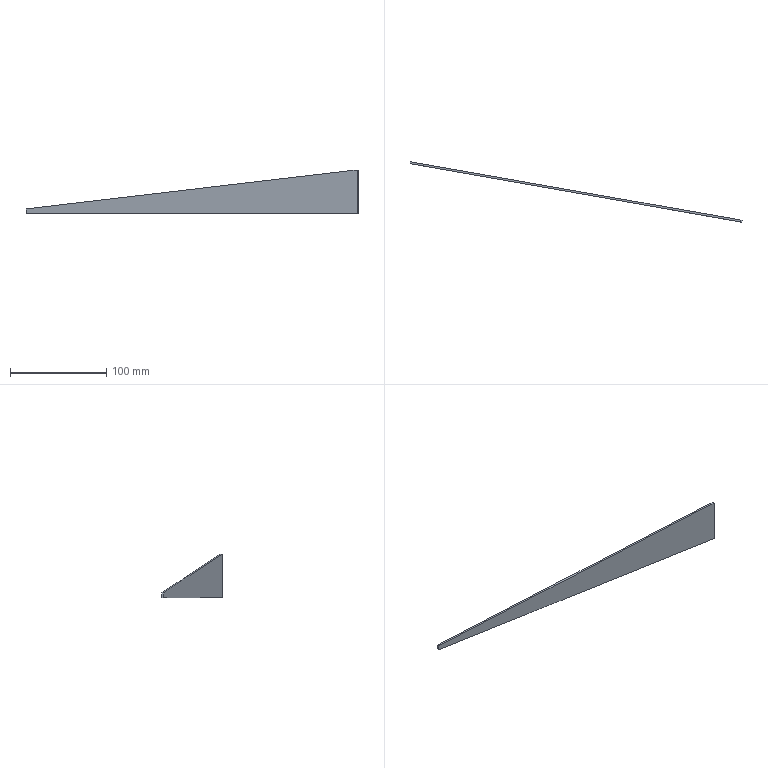Part | SolidWorks | features Extrusion 1 | 1 solid | 7 faces | box 345.03 x 62.746 x 45 mm | volume 17700 mm3 | plane 7
STEP:
#1=CARTESIAN_POINT('',(-12.484,1.186,10.));
#2=VERTEX_POINT('',#1);
#3=CARTESIAN_POINT('',(-357.166,61.963,10.));
#4=VERTEX_POINT('',#3);
#5=CARTESIAN_POINT('',(-12.484,1.186,10.));
#6=DIRECTION('',(-0.9848,0.1736,0.));
#7=VECTOR('',#6,1000.);
#8=LINE('',#5,#7);
#9=EDGE_CURVE('',#2,#4,#8,.T.);
#10=ORIENTED_EDGE('',*,*,#9,.T.);
#11=CARTESIAN_POINT('',(-356.819,63.932,10.));
#12=VERTEX_POINT('',#11);
#13=CARTESIAN_POINT('',(-356.819,63.932,10.));
#14=DIRECTION('',(-0.1736,-0.9848,0.));
#15=VECTOR('',#14,1000.);
#16=LINE('',#13,#15);
#17=EDGE_CURVE('',#12,#4,#16,.T.);
#18=ORIENTED_EDGE('',*,*,#17,.F.);
#19=CARTESIAN_POINT('',(-12.136,3.155,10.));
#20=VERTEX_POINT('',#19);
#21=CARTESIAN_POINT('',(-12.136,3.155,10.));
#22=DIRECTION('',(-0.9848,0.1736,0.));
#23=VECTOR('',#22,1000.);
#24=LINE('',#21,#23);
#25=EDGE_CURVE('',#20,#12,#24,.T.);
#26=ORIENTED_EDGE('',*,*,#25,.F.);
#27=CARTESIAN_POINT('',(-12.136,3.155,10.));
#28=DIRECTION('',(-0.1736,-0.9848,0.));
#29=VECTOR('',#28,1000.);
#30=LINE('',#27,#29);
#31=EDGE_CURVE('',#20,#2,#30,.T.);
#32=ORIENTED_EDGE('',*,*,#31,.T.);
#33=EDGE_LOOP('',(#10,#18,#26,#32));
#34=FACE_OUTER_BOUND('',#33,.T.);
#35=CARTESIAN_POINT('',(-12.136,3.155,10.));
#36=DIRECTION('',(0.,0.,1.));
#37=DIRECTION('',(1.,0.,0.));
#38=AXIS2_PLACEMENT_3D('',#35,#36,#37);
#39=PLANE('',#38);
#40=ADVANCED_FACE('',(#34),#39,.F.);
#41=CARTESIAN_POINT('',(-357.166,61.963,15.));
#42=VERTEX_POINT('',#41);
#43=CARTESIAN_POINT('',(-357.166,61.963,10.));
#44=DIRECTION('',(0.,0.,1.));
#45=VECTOR('',#44,1000.);
#46=LINE('',#43,#45);
#47=EDGE_CURVE('',#4,#42,#46,.T.);
#48=ORIENTED_EDGE('',*,*,#47,.T.);
#49=CARTESIAN_POINT('',(-356.819,63.932,15.));
#50=VERTEX_POINT('',#49);
#51=CARTESIAN_POINT('',(-356.819,63.932,15.));
#52=DIRECTION('',(-0.1736,-0.9848,0.));
#53=VECTOR('',#52,1000.);
#54=LINE('',#51,#53);
#55=EDGE_CURVE('',#50,#42,#54,.T.);
#56=ORIENTED_EDGE('',*,*,#55,.F.);
#57=CARTESIAN_POINT('',(-356.819,63.932,10.));
#58=DIRECTION('',(0.,0.,1.));
#59=VECTOR('',#58,1000.);
#60=LINE('',#57,#59);
#61=EDGE_CURVE('',#12,#50,#60,.T.);
#62=ORIENTED_EDGE('',*,*,#61,.F.);
#63=ORIENTED_EDGE('',*,*,#17,.T.);
#64=EDGE_LOOP('',(#48,#56,#62,#63));
#65=FACE_OUTER_BOUND('',#64,.T.);
#66=CARTESIAN_POINT('',(-356.819,63.932,10.));
#67=DIRECTION('',(0.9848,-0.1736,0.));
#68=DIRECTION('',(0.1736,0.9848,0.));
#69=AXIS2_PLACEMENT_3D('',#66,#67,#68);
#70=PLANE('',#69);
#71=ADVANCED_FACE('',(#65),#70,.F.);
#72=CARTESIAN_POINT('',(-17.408,2.054,55.));
#73=VERTEX_POINT('',#72);
#74=CARTESIAN_POINT('',(-357.166,61.963,15.));
#75=DIRECTION('',(0.9783,-0.1725,0.1152));
#76=VECTOR('',#75,1000.);
#77=LINE('',#74,#76);
#78=EDGE_CURVE('',#42,#73,#77,.T.);
#79=ORIENTED_EDGE('',*,*,#78,.T.);
#80=CARTESIAN_POINT('',(-17.06,4.024,55.));
#81=VERTEX_POINT('',#80);
#82=CARTESIAN_POINT('',(-17.06,4.024,55.));
#83=DIRECTION('',(-0.1736,-0.9848,0.));
#84=VECTOR('',#83,1000.);
#85=LINE('',#82,#84);
#86=EDGE_CURVE('',#81,#73,#85,.T.);
#87=ORIENTED_EDGE('',*,*,#86,.F.);
#88=CARTESIAN_POINT('',(-356.819,63.932,15.));
#89=DIRECTION('',(0.9783,-0.1725,0.1152));
#90=VECTOR('',#89,1000.);
#91=LINE('',#88,#90);
#92=EDGE_CURVE('',#50,#81,#91,.T.);
#93=ORIENTED_EDGE('',*,*,#92,.F.);
#94=ORIENTED_EDGE('',*,*,#55,.T.);
#95=EDGE_LOOP('',(#79,#87,#93,#94));
#96=FACE_OUTER_BOUND('',#95,.T.);
#97=CARTESIAN_POINT('',(-356.819,63.932,15.));
#98=DIRECTION('',(0.1134,-0.02,-0.9933));
#99=DIRECTION('',(-0.9935,0.,-0.1134));
#100=AXIS2_PLACEMENT_3D('',#97,#98,#99);
#101=PLANE('',#100);
#102=ADVANCED_FACE('',(#96),#101,.F.);
#103=CARTESIAN_POINT('',(-12.484,1.186,55.));
#104=VERTEX_POINT('',#103);
#105=CARTESIAN_POINT('',(-12.484,1.186,55.));
#106=DIRECTION('',(0.9848,-0.1736,0.));
#107=VECTOR('',#106,1000.);
#108=LINE('',#105,#107);
#109=EDGE_CURVE('',#73,#104,#108,.T.);
#110=ORIENTED_EDGE('',*,*,#109,.T.);
#111=CARTESIAN_POINT('',(-12.136,3.155,55.));
#112=VERTEX_POINT('',#111);
#113=CARTESIAN_POINT('',(-12.136,3.155,55.));
#114=DIRECTION('',(-0.1736,-0.9848,0.));
#115=VECTOR('',#114,1000.);
#116=LINE('',#113,#115);
#117=EDGE_CURVE('',#112,#104,#116,.T.);
#118=ORIENTED_EDGE('',*,*,#117,.F.);
#119=CARTESIAN_POINT('',(-12.136,3.155,55.));
#120=DIRECTION('',(0.9848,-0.1736,0.));
#121=VECTOR('',#120,1000.);
#122=LINE('',#119,#121);
#123=EDGE_CURVE('',#81,#112,#122,.T.);
#124=ORIENTED_EDGE('',*,*,#123,.F.);
#125=ORIENTED_EDGE('',*,*,#86,.T.);
#126=EDGE_LOOP('',(#110,#118,#124,#125));
#127=FACE_OUTER_BOUND('',#126,.T.);
#128=CARTESIAN_POINT('',(-12.136,3.155,55.));
#129=DIRECTION('',(0.,0.,-1.));
#130=DIRECTION('',(-1.,0.,0.));
#131=AXIS2_PLACEMENT_3D('',#128,#129,#130);
#132=PLANE('',#131);
#133=ADVANCED_FACE('',(#127),#132,.F.);
#134=CARTESIAN_POINT('',(-12.484,1.186,10.));
#135=DIRECTION('',(0.,0.,-1.));
#136=VECTOR('',#135,1000.);
#137=LINE('',#134,#136);
#138=EDGE_CURVE('',#104,#2,#137,.T.);
#139=ORIENTED_EDGE('',*,*,#138,.T.);
#140=ORIENTED_EDGE('',*,*,#31,.F.);
#141=CARTESIAN_POINT('',(-12.136,3.155,10.));
#142=DIRECTION('',(0.,0.,-1.));
#143=VECTOR('',#142,1000.);
#144=LINE('',#141,#143);
#145=EDGE_CURVE('',#112,#20,#144,.T.);
#146=ORIENTED_EDGE('',*,*,#145,.F.);
#147=ORIENTED_EDGE('',*,*,#117,.T.);
#148=EDGE_LOOP('',(#139,#140,#146,#147));
#149=FACE_OUTER_BOUND('',#148,.T.);
#150=CARTESIAN_POINT('',(-12.136,3.155,10.));
#151=DIRECTION('',(-0.9848,0.1736,0.));
#152=DIRECTION('',(-0.1736,-0.9848,0.));
#153=AXIS2_PLACEMENT_3D('',#150,#151,#152);
#154=PLANE('',#153);
#155=ADVANCED_FACE('',(#149),#154,.F.);
#156=ORIENTED_EDGE('',*,*,#25,.T.);
#157=ORIENTED_EDGE('',*,*,#61,.T.);
#158=ORIENTED_EDGE('',*,*,#92,.T.);
#159=ORIENTED_EDGE('',*,*,#123,.T.);
#160=ORIENTED_EDGE('',*,*,#145,.T.);
#161=EDGE_LOOP('',(#156,#157,#158,#159,#160));
#162=FACE_OUTER_BOUND('',#161,.T.);
#163=CARTESIAN_POINT('',(0.1736,0.9848,0.));
#164=DIRECTION('',(0.1736,0.9848,0.));
#165=DIRECTION('',(-0.9848,0.1736,0.));
#166=AXIS2_PLACEMENT_3D('',#163,#164,#165);
#167=PLANE('',#166);
#168=ADVANCED_FACE('',(#162),#167,.T.);
#169=ORIENTED_EDGE('',*,*,#9,.F.);
#170=ORIENTED_EDGE('',*,*,#138,.F.);
#171=ORIENTED_EDGE('',*,*,#109,.F.);
#172=ORIENTED_EDGE('',*,*,#78,.F.);
#173=ORIENTED_EDGE('',*,*,#47,.F.);
#174=EDGE_LOOP('',(#169,#170,#171,#172,#173));
#175=FACE_OUTER_BOUND('',#174,.T.);
#176=CARTESIAN_POINT('',(-0.1736,-0.9848,0.));
#177=DIRECTION('',(0.1736,0.9848,0.));
#178=DIRECTION('',(-0.9848,0.1736,0.));
#179=AXIS2_PLACEMENT_3D('',#176,#177,#178);
#180=PLANE('',#179);
#181=ADVANCED_FACE('',(#175),#180,.F.);
#182=CLOSED_SHELL('',(#40,#71,#102,#133,#155,#168,#181));
#183=MANIFOLD_SOLID_BREP('',#182);
#184=CARTESIAN_POINT('',(0.,0.,0.));
#185=DIRECTION('',(0.,0.,1.));
#186=DIRECTION('',(1.,0.,0.));
#187=AXIS2_PLACEMENT_3D('',#184,#185,#186);
#188=(LENGTH_UNIT()NAMED_UNIT(*)SI_UNIT(.MILLI.,.METRE.));
#189=UNCERTAINTY_MEASURE_WITH_UNIT(LENGTH_MEASURE(0.00001),#188,'','');
#190=(NAMED_UNIT(*)PLANE_ANGLE_UNIT()SI_UNIT($,.RADIAN.));
#191=(NAMED_UNIT(*)SI_UNIT($,.STERADIAN.)SOLID_ANGLE_UNIT());
#192=(GEOMETRIC_REPRESENTATION_CONTEXT(3)GLOBAL_UNCERTAINTY_ASSIGNED_CONTEXT((#189))GLOBAL_UNIT_ASSIGNED_CONTEXT((#188,#190,#191))REPRESENTATION_CONTEXT('',''));
#193=ADVANCED_BREP_SHAPE_REPRESENTATION('',(#183,#187),#192);